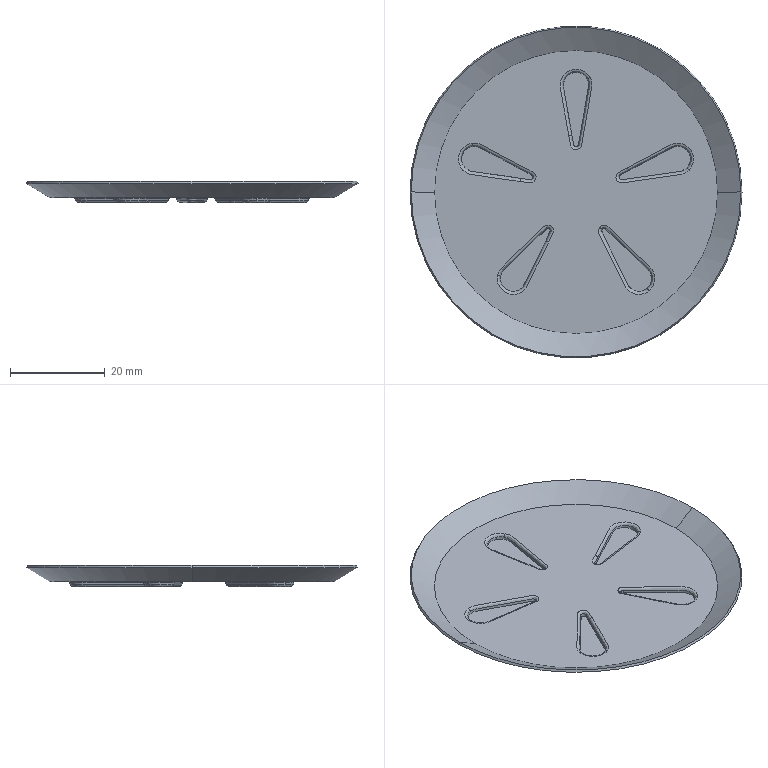Part | SolidWorks | features BaseBody 1 | 1 solid | 70 faces | box 70 x 70 x 4.429 mm | volume 2054 mm3 | spline 50 | plane 12 | cone 6 | torus 2